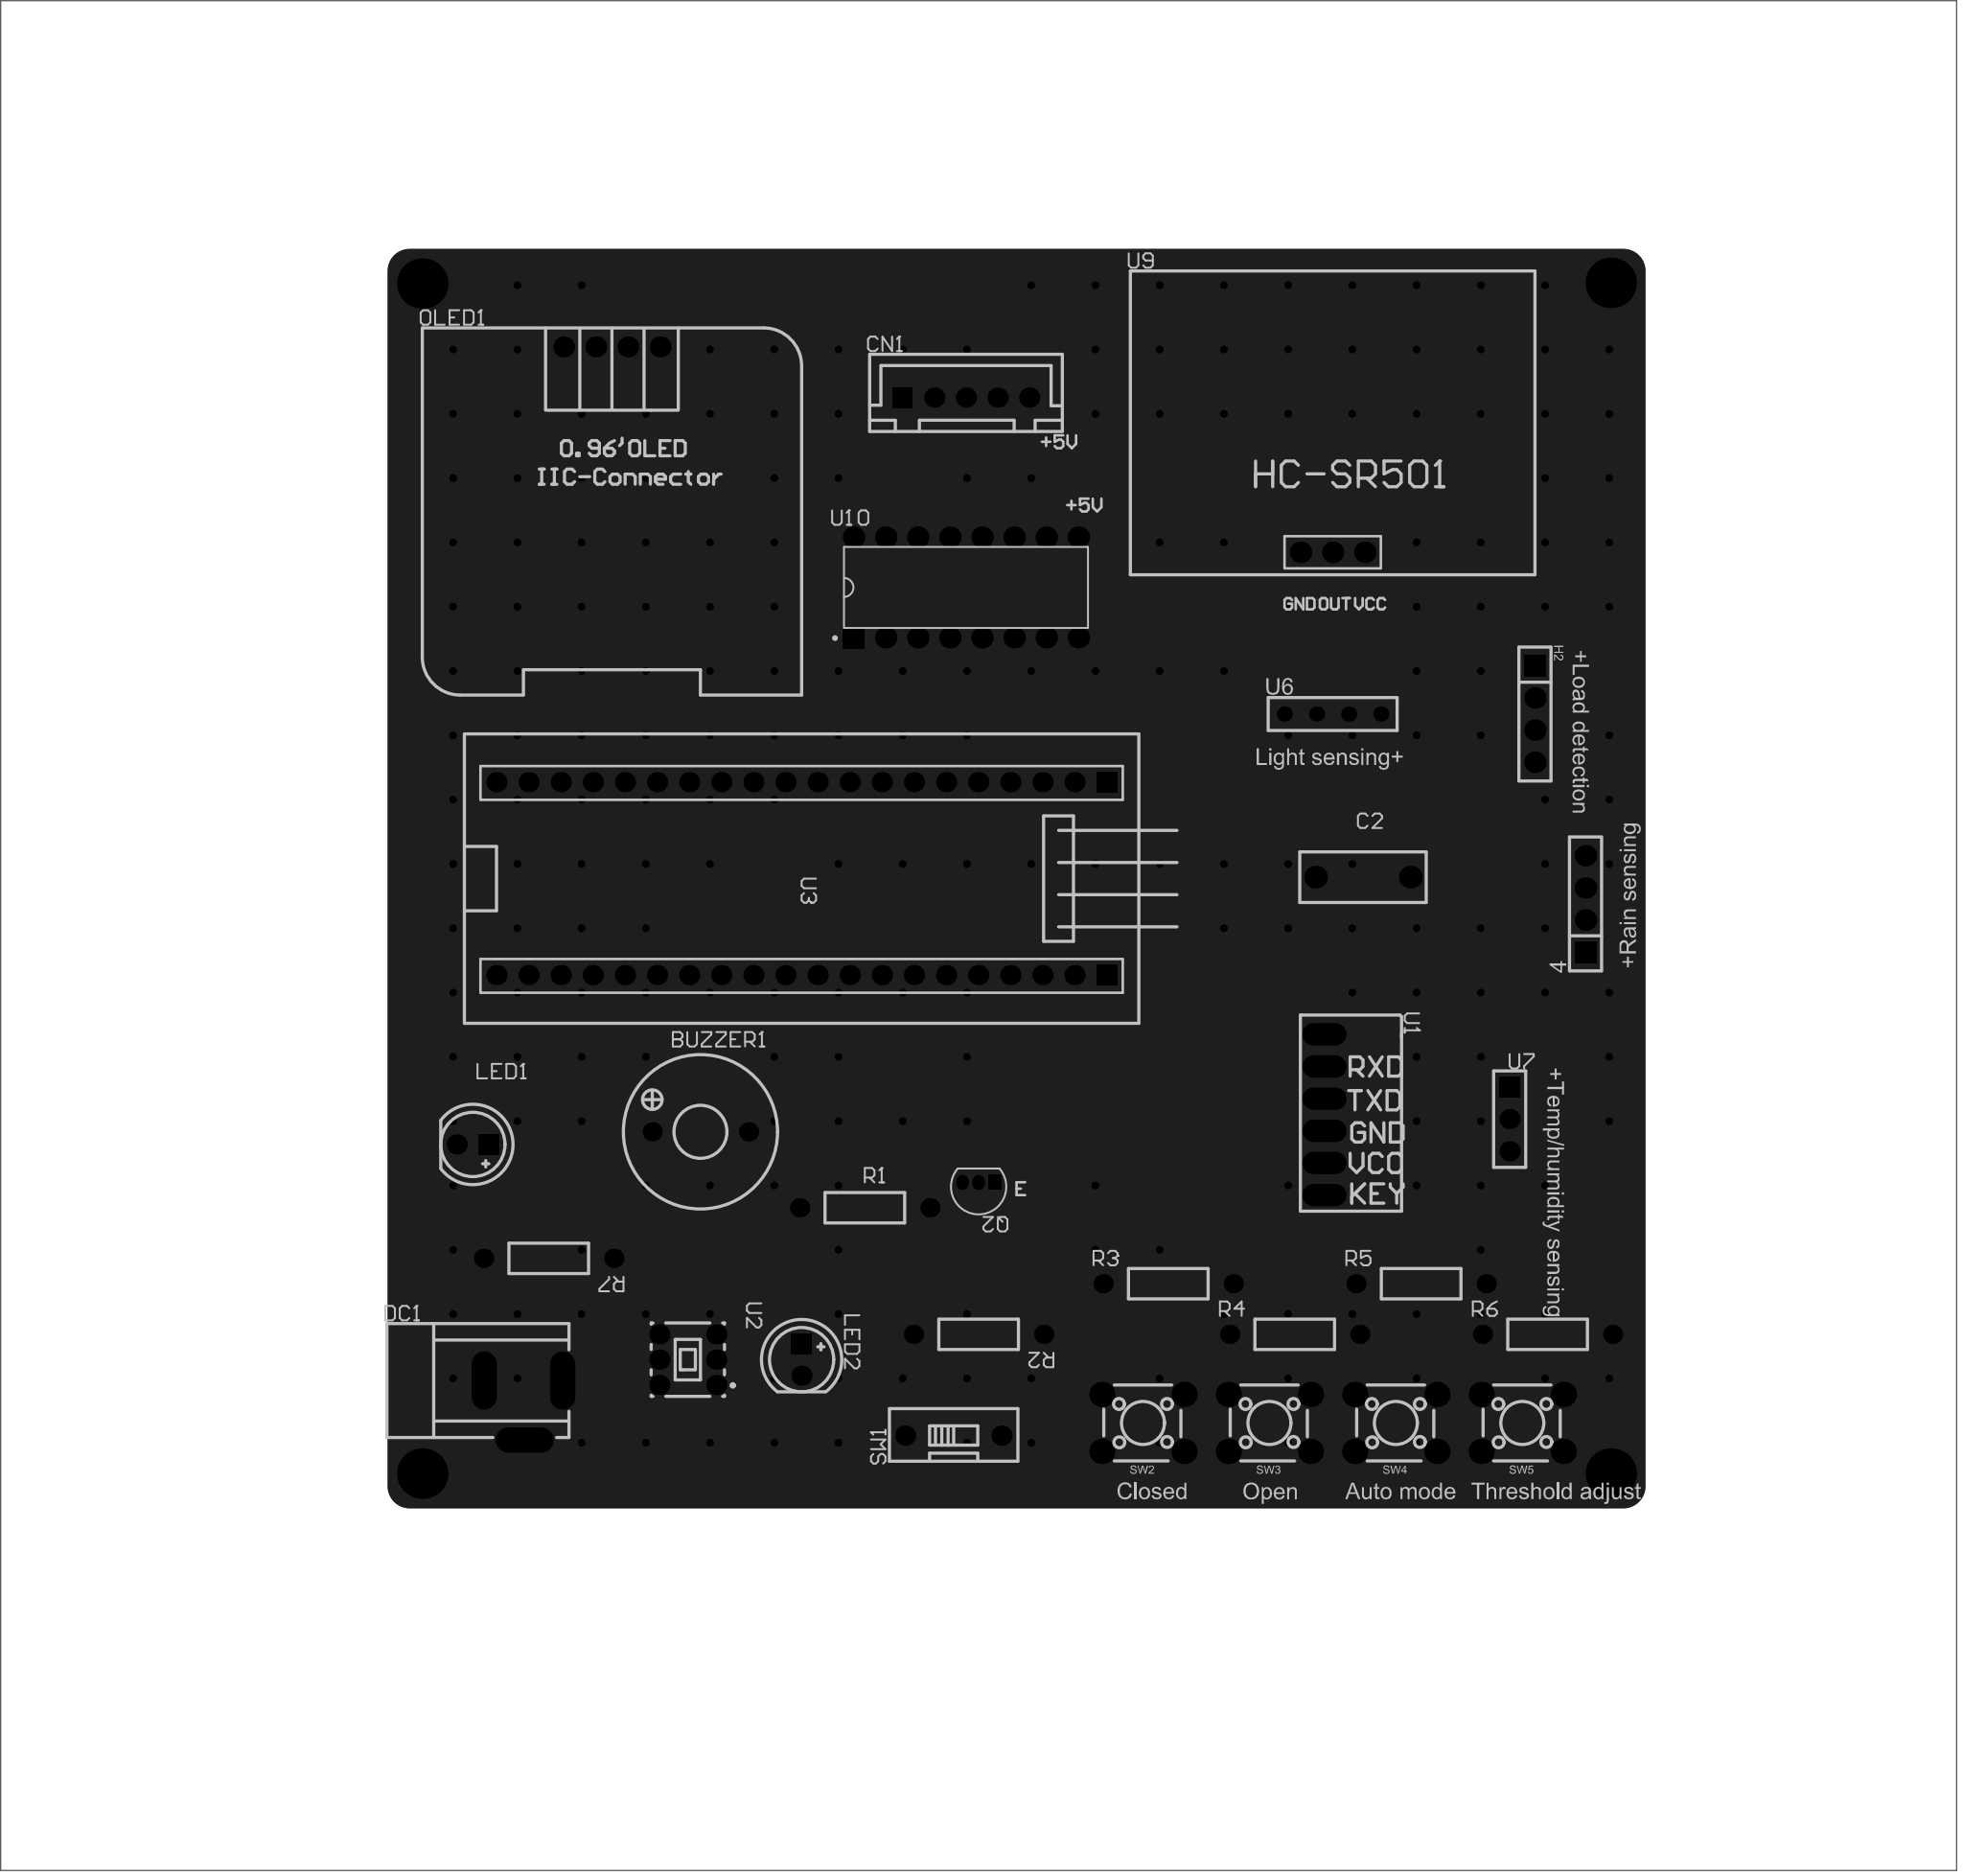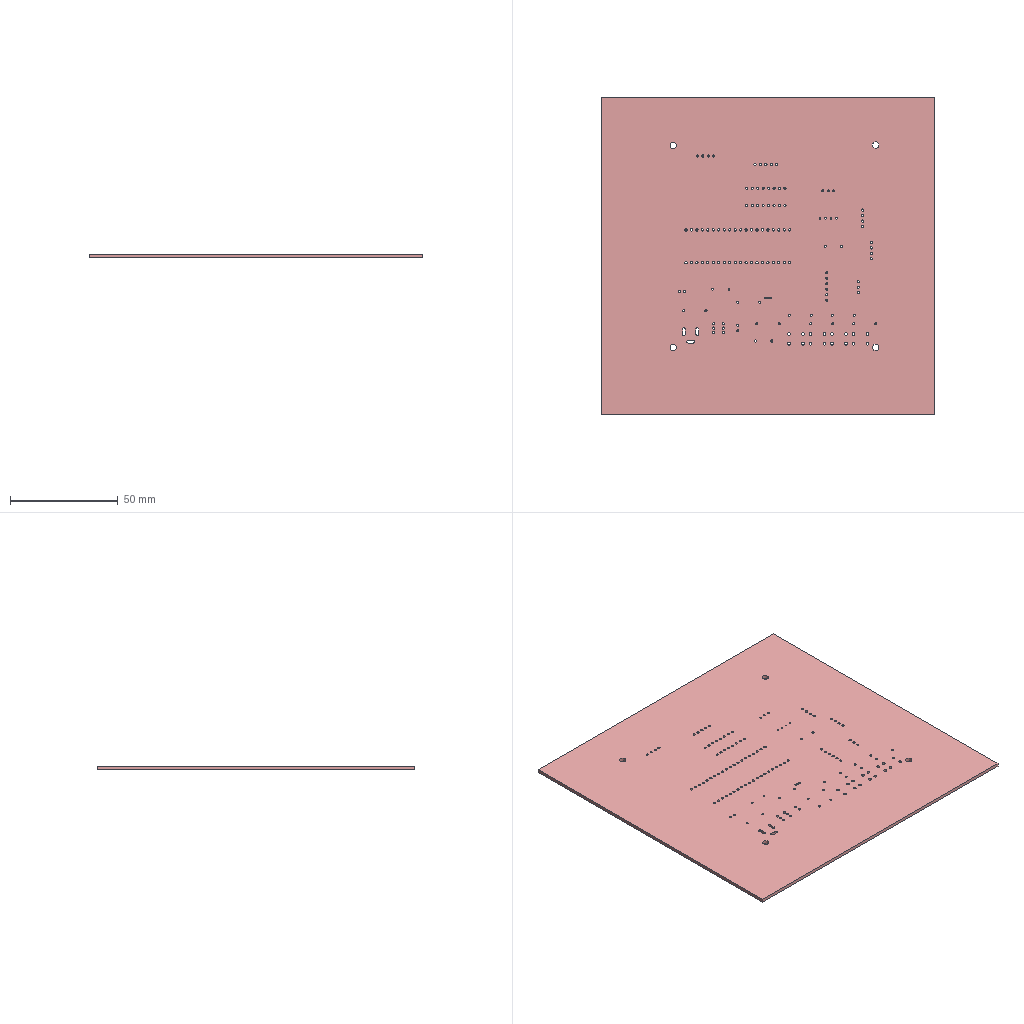Circuit board layout | Altium Designer | box 154.7 x 147.7 x 1.6 mm
Layer stack:
# Altium Designer layer stack of  (unit mm; dielectric type: 0 none, 1 core, 2 prepreg, 3 surface material)
index,name,kind,layer,copper_thickness_mm,dielectric_type,dielectric_thickness_mm,dielectric_material,dielectric_constant
0,Top Paste Mask Layer,other,,,,,,
1,Top Silkscreen Layer,other,,,,,,
2,Top Solder Mask Layer,dielectric,,,3,0.01,,3.3
3,Top Layer,copper,Top Layer,0.035,,,,
4,Dielectric1,dielectric,,,3,1.51,FR4,4.5
5,Bottom Layer,copper,Bottom Layer,0.035,,,,
6,Bottom Solder Mask Layer,dielectric,,,3,0.01,,3.3
7,Bottom Silkscreen Layer,other,,,,,,
8,Bottom Paste Mask Layer,other,,,,,,
# drill layer pairs: low layer,high layer
drill_pair,Top Layer,Bottom Layer
Part placement:
Designator,Comment,Layer,Footprint,Center-X(mm),Center-Y(mm),Rotation
4,,TopLayer,HDR-TH_4P-P2.54-V-F,195.2,146.2,90
CN1,HX-XH2.54-5PZZ,TopLayer,CONN-TH_5P-P2.50_ZX-XH2.54-5PZZ,146.2,186.2,0
DC1,DC005,TopLayer,DC-IN-TH_DC005,111.2,106.2,0
H2,,TopLayer,HDR-TH_4P-P2.54-V-F,191.2,161.2,270
LED1,,TopLayer,LED-TH_5mm,107.2,127.2,180
LED2,,TopLayer,LED-TH_5mm,133.2,110.2,270
OLED1,,TopLayer,0.96OLED_4P,118.2,190.2,0
R1,1K,TopLayer,Res_1/4W,138.2,122.2,0
R2,10kΩ,TopLayer,Res_1/4W,147.2,112.2,180
R3,10kΩ,TopLayer,Res_1/4W,162.2,116.2,0
R4,10kΩ,TopLayer,Res_1/4W,172.2,112.2,0
R5,10kΩ,TopLayer,Res_1/4W,182.2,116.2,0
R6,10kΩ,TopLayer,Res_1/4W,192.2,112.2,0
R7,1K,TopLayer,Res_1/4W,113.2,118.2,180
SW1,DIP switch,TopLayer,SW-TH_DSWB01LHGET,145.2,104.2,90
SW2,Tact switch,TopLayer,KEY-TH_4P-L6.0-W6.0-P4.50-LS6.50,160.2,105.2,180
SW3,Tact switch,TopLayer,KEY-TH_4P-L6.0-W6.0-P4.50-LS6.50,170.2,105.2,180
SW4,Tact switch,TopLayer,KEY-TH_4P-L6.0-W6.0-P4.50-LS6.50,180.2,105.2,180
SW5,Tact switch,TopLayer,KEY-TH_4P-L6.0-W6.0-P4.50-LS6.50,190.2,105.2,180
U1,HC05,TopLayer,HC05,174.553,129.549,270
U3,STM32F103C8T6,TopLayer,STM32F103C8T6核心板,133.2,148.2,270
U6,,TopLayer,HDR-TH_4P-P2.54_342-40-104-00-592000,175.2,161.2,0
U9,HC-SR501 human infrared sensor,TopLayer,大闸蟹-HC-SR501人体红外传感器,175.202,173.978,0
U10,ULN2003AN(XBLW),TopLayer,PDIP-16_L19.3-W6.4-P2.54-LS7.9-BL,146.2,171.2,0
BUZZER1,3kHz,TopLayer,BUZZER,125.2,128.2,90
Q2,S8050,TopLayer,TO-92-3_L4.5-W3.5-P1.27-L,147.2,124.2,180
C2,10uF,TopLayer,CAP-TH_L10.0-W4.0-P7.50-D0.6-1,177.599,148.312,180
U2,Self-lock switch,TopLayer,SW-TH_6P-L5.8-W5.8-P2.00-LS4.5-TR,124.2,110.2,270
U7,,TopLayer,HDR-TH_3P-P2.54-V-M-B,189.2,129.2,90
Pad and via stacks:
# Altium Designer via and pad stacks of  (unit mm). Each distinct definition once, with the count of objects using it.
# via: kind,start_layer,end_layer,hole_mm,diameter_mm,mode(0 simple;1 top-mid-bottom;2 full stack),diameter_per_layer,count,example_net
# pad: kind,layer,hole_mm,hole_type(0 round;1 square;2 slot),plating,top_size,top_shape(1 round;2 rect;3 octagon;9 rounded rect),mid_size,bottom_size,mode,footprint,size_per_layer,count,example
pad,Multi-Layer,3,0,plated,4x4,1,4x4,4x4,0,,,4,1
pad,Multi-Layer,1.1,0,plated,1.7x1.7,2,1.7x1.7,1.7x1.7,0,HDR-TH_4P-P2.54-V-F,,2,4.1
pad,Multi-Layer,1.1,0,plated,1.7x1.7,1,1.7x1.7,1.7x1.7,0,HDR-TH_4P-P2.54-V-F,,6,4.2
pad,Multi-Layer,1.1,0,plated,1.6x1.6,1,1.6x1.6,1.6x1.6,0,CONN-TH_5P-P2.50_ZX-XH2.54-5PZZ,,4,CN1.4
pad,Multi-Layer,1.1,0,plated,1.524x1.6,2,1.524x1.6,1.524x1.6,0,CONN-TH_5P-P2.50_ZX-XH2.54-5PZZ,,1,CN1.1
pad,Multi-Layer,1.2,2,plated,2x4.6,1,2x4.6,2x4.6,0,DC-IN-TH_DC005,,2,DC1.1
pad,Multi-Layer,1.2,2,plated,4.6x2,1,4.6x2,4.6x2,0,DC-IN-TH_DC005,,1,DC1.3
pad,Multi-Layer,1,0,plated,1.6x1.6,2,1.6x1.6,1.6x1.6,0,LED-TH_5mm,,2,LED1.1
pad,Multi-Layer,1,0,plated,1.6x1.6,1,1.6x1.6,1.6x1.6,0,LED-TH_5mm,,2,LED1.2
pad,Multi-Layer,1,0,plated,1.65x1.65,1,1.65x1.65,1.65x1.65,0,0.96OLED_4P,,4,OLED1.4
pad,Multi-Layer,1,0,plated,1.524x1.524,1,1.524x1.524,1.524x1.524,0,Res_1/4W,,14,R1.1
pad,Multi-Layer,1,0,plated,1.6x1.6,1,1.6x1.6,1.6x1.6,0,SW-TH_DSWB01LHGET,,2,SW1.2
pad,Multi-Layer,1.3,0,plated,2x2,1,2x2,2x2,0,KEY-TH_4P-L6.0-W6.0-P4.50-LS6.50,,16,SW2.4
pad,Multi-Layer,1.016,0,plated,1.778x3.5,1,1.778x3.5,1.778x3.5,0,HC05,,6,U1.6
pad,Multi-Layer,1.049,0,plated,1.6x1.6,2,1.6x1.6,1.6x1.6,0,STM32F103C8T6\u00BA\u00CB\u00D0\u00C4\u00B0\u00E5,,2,U3.1
pad,Multi-Layer,1.049,0,plated,1.6x1.6,1,1.6x1.6,1.6x1.6,0,STM32F103C8T6\u00BA\u00CB\u00D0\u00C4\u00B0\u00E5,,38,U3.2
pad,Multi-Layer,0.7,0,plated,1.2x1.2,1,1.2x1.2,1.2x1.2,0,HDR-TH_4P-P2.54_342-40-104-00-592000,,4,U6.1
pad,Multi-Layer,0.9,0,plated,1.7x1.7,1,1.7x1.7,1.7x1.7,0,\u00B4\u00F3\u00D5\u00A2\u00D0\u00B7-HC-SR501\u00C8\u00CB\u00CC\u00E5\u00BA\u00EC\u00CD\u00E2\u00B4\u00AB\u00B8\u00D0\u00C6\u00F7,,2,U9.3
pad,Multi-Layer,0.9,2,plated,1.7x1.7,1,1.7x1.7,1.7x1.7,0,\u00B4\u00F3\u00D5\u00A2\u00D0\u00B7-HC-SR501\u00C8\u00CB\u00CC\u00E5\u00BA\u00EC\u00CD\u00E2\u00B4\u00AB\u00B8\u00D0\u00C6\u00F7,,1,U9.1
pad,Multi-Layer,1,0,plated,1.7x1.7,2,1.7x1.7,1.7x1.7,0,PDIP-16_L19.3-W6.4-P2.54-LS7.9-BL,,1,U10.1
pad,Multi-Layer,1,0,plated,1.7x1.7,1,1.7x1.7,1.7x1.7,0,PDIP-16_L19.3-W6.4-P2.54-LS7.9-BL,,15,U10.2
pad,Multi-Layer,0.762,0,plated,1.524x1.524,1,1.524x1.524,1.524x1.524,0,BUZZER,,2,BUZZER1.1
pad,Multi-Layer,0.7,2,plated,1x1.2,2,1x1.2,1x1.2,0,TO-92-3_L4.5-W3.5-P1.27-L,,1,Q2.1
pad,Multi-Layer,0.7,2,plated,1x1.2,1,1x1.2,1x1.2,0,TO-92-3_L4.5-W3.5-P1.27-L,,2,Q2.2
pad,Multi-Layer,1,0,plated,1.8x1.8,1,1.8x1.8,1.8x1.8,0,CAP-TH_L10.0-W4.0-P7.50-D0.6-1,,2,C2.2
pad,Multi-Layer,1.1,0,plated,1.6x1.6,1,1.6x1.6,1.6x1.6,0,SW-TH_6P-L5.8-W5.8-P2.00-LS4.5-TR,,6,U2.6
pad,Multi-Layer,1.02,0,plated,1.6x1.6,2,1.6x1.6,1.6x1.6,0,HDR-TH_3P-P2.54-V-M-B,,1,U7.1
pad,Multi-Layer,1.02,0,plated,1.6x1.6,1,1.6x1.6,1.6x1.6,0,HDR-TH_3P-P2.54-V-M-B,,2,U7.2
via,Top Layer,Bottom Layer,0.3048,0.61,0,,225,GND
Copper pours:
name,layer,net,type(0 solid;1 hatched;2 none)
Bottom Layer-GND,Bottom Layer,GND,0
Top Layer-GND,Top Layer,GND,0
Design rules, without the lines most boards share:
# Altium Designer design rules of  (exported by Altium Designer, unit mm)
# columns: name | kind | enabled | priority | scope1 | scope2 | descriptor | typed fields (field=value)
power | 2 | enabled | 2 | (InNet('+5V') OR InNet('GND') OR InNet('+3.3V') OR InNet('IN_5V')) | All | Width Constraint (Min=10mil) (Max=100mil) (Preferred=20mil) ((InNet('+5V') OR InNet('GND') OR InNet('+3.3V') OR InNet('IN_5V'))) |
copperThickness1oz_2 | 2 | enabled | 3 | All | All | Width Constraint (Min=5mil) (Max=100mil) (Preferred=10mil) (All) |
copperRegion_Top Layer | 20 | enabled | 1 | (InNet('GND')) And OnLayer('Top Layer') | All | Polygon Connect Rule(Relief Connect )(Conductor Width=10mil) (Relief Angle=90 Angle) (Entries=4) (Air Gap Width=10mil) ((InNet('GND')) And OnLayer('Top Layer')),(All) | connect_style(0=relief,1=direct,2=none)=0 relief_conductor_width=0.254 relief_entries=4
copperRegion_Bottom Layer | 20 | enabled | 2 | (InNet('GND')) And OnLayer('Bottom Layer') | All | Polygon Connect Rule(Relief Connect )(Conductor Width=10mil) (Relief Angle=90 Angle) (Entries=4) (Air Gap Width=10mil) ((InNet('GND')) And OnLayer('Bottom Layer')),(All) | connect_style(0=relief,1=direct,2=none)=0 relief_conductor_width=0.254 relief_entries=4
copperRegion | 20 | enabled | 3 | (InNet('GND')) | All | Polygon Connect Rule(Direct Connect )(Conductor Width=10mil) (Relief Angle=90 Angle) (Entries=4) (Air Gap Width=10mil) ((InNet('GND'))),(All) | connect_style(0=relief,1=direct,2=none)=1 relief_conductor_width=0.254 relief_entries=4